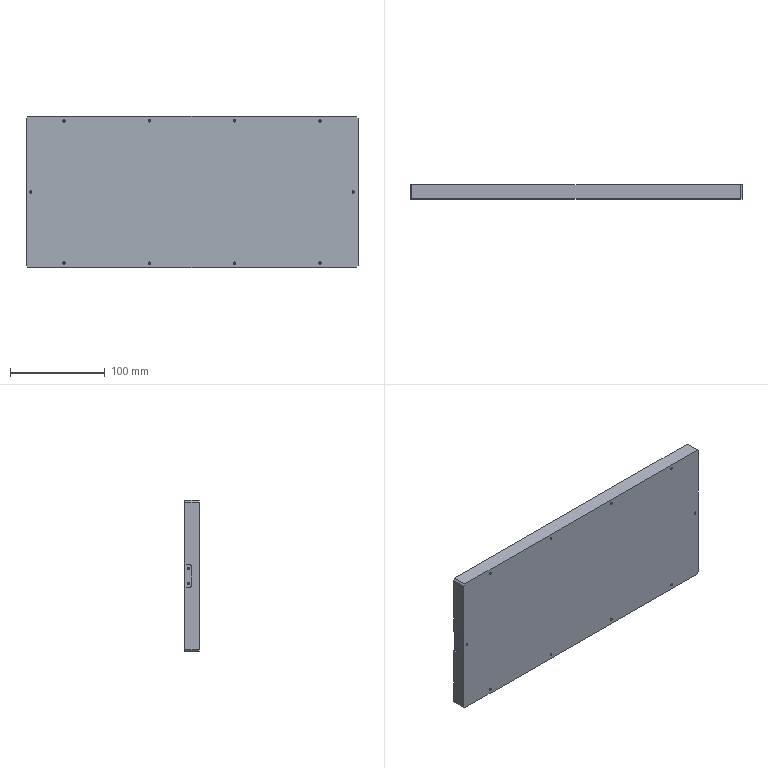Part | SolidWorks | features BaseBody 1 | 1 solid | 110 faces | box 350 x 15 x 160 mm | volume 836059 mm3 | cylinder 48 | cone 44 | plane 18 | commonest cylinder face diameters 2.5 x28 6 x12 10 x8